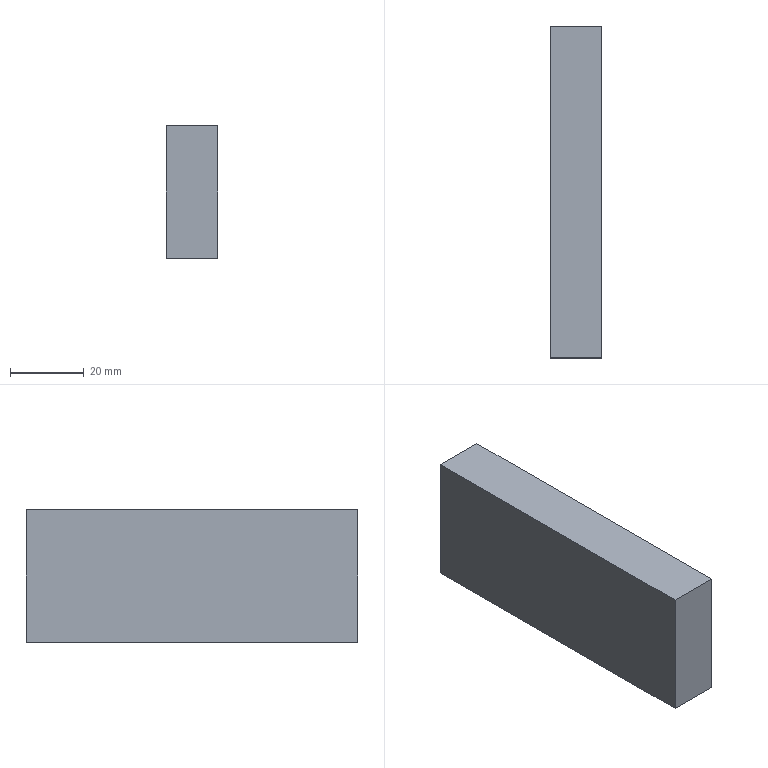Part | NX | features solid 2 | 1 solid | 6 faces | box 14 x 90 x 36 mm | volume 45360 mm3 | plane 6
STEP:
#1=CARTESIAN_POINT('',(300.,335.,9.));
#2=VERTEX_POINT('',#1);
#3=CARTESIAN_POINT('',(300.,245.,9.));
#4=VERTEX_POINT('',#3);
#5=CARTESIAN_POINT('',(300.,335.,9.));
#6=DIRECTION('',(0.,-1.,0.));
#7=VECTOR('',#6,1000.);
#8=LINE('',#5,#7);
#9=EDGE_CURVE('',#2,#4,#8,.T.);
#10=ORIENTED_EDGE('',*,*,#9,.T.);
#11=CARTESIAN_POINT('',(300.,245.,45.));
#12=VERTEX_POINT('',#11);
#13=CARTESIAN_POINT('',(300.,245.,45.));
#14=DIRECTION('',(0.,0.,-1.));
#15=VECTOR('',#14,1000.);
#16=LINE('',#13,#15);
#17=EDGE_CURVE('',#12,#4,#16,.T.);
#18=ORIENTED_EDGE('',*,*,#17,.F.);
#19=CARTESIAN_POINT('',(300.,335.,45.));
#20=VERTEX_POINT('',#19);
#21=CARTESIAN_POINT('',(300.,335.,45.));
#22=DIRECTION('',(0.,-1.,0.));
#23=VECTOR('',#22,1000.);
#24=LINE('',#21,#23);
#25=EDGE_CURVE('',#20,#12,#24,.T.);
#26=ORIENTED_EDGE('',*,*,#25,.F.);
#27=CARTESIAN_POINT('',(300.,335.,45.));
#28=DIRECTION('',(0.,0.,-1.));
#29=VECTOR('',#28,1000.);
#30=LINE('',#27,#29);
#31=EDGE_CURVE('',#20,#2,#30,.T.);
#32=ORIENTED_EDGE('',*,*,#31,.T.);
#33=EDGE_LOOP('',(#10,#18,#26,#32));
#34=FACE_BOUND('',#33,.T.);
#35=CARTESIAN_POINT('',(300.,335.,45.));
#36=DIRECTION('',(1.,0.,0.));
#37=DIRECTION('',(0.,0.,-1.));
#38=AXIS2_PLACEMENT_3D('',#35,#36,#37);
#39=PLANE('',#38);
#40=ADVANCED_FACE('',(#34),#39,.F.);
#41=CARTESIAN_POINT('',(314.,245.,9.));
#42=VERTEX_POINT('',#41);
#43=CARTESIAN_POINT('',(314.,245.,9.));
#44=DIRECTION('',(-1.,0.,0.));
#45=VECTOR('',#44,1000.);
#46=LINE('',#43,#45);
#47=EDGE_CURVE('',#42,#4,#46,.T.);
#48=ORIENTED_EDGE('',*,*,#47,.F.);
#49=CARTESIAN_POINT('',(314.,245.,45.));
#50=VERTEX_POINT('',#49);
#51=CARTESIAN_POINT('',(314.,245.,45.));
#52=DIRECTION('',(0.,0.,-1.));
#53=VECTOR('',#52,1000.);
#54=LINE('',#51,#53);
#55=EDGE_CURVE('',#50,#42,#54,.T.);
#56=ORIENTED_EDGE('',*,*,#55,.F.);
#57=CARTESIAN_POINT('',(314.,245.,45.));
#58=DIRECTION('',(-1.,0.,0.));
#59=VECTOR('',#58,1000.);
#60=LINE('',#57,#59);
#61=EDGE_CURVE('',#50,#12,#60,.T.);
#62=ORIENTED_EDGE('',*,*,#61,.T.);
#63=ORIENTED_EDGE('',*,*,#17,.T.);
#64=EDGE_LOOP('',(#48,#56,#62,#63));
#65=FACE_BOUND('',#64,.T.);
#66=CARTESIAN_POINT('',(314.,245.,45.));
#67=DIRECTION('',(0.,-1.,0.));
#68=DIRECTION('',(0.,0.,-1.));
#69=AXIS2_PLACEMENT_3D('',#66,#67,#68);
#70=PLANE('',#69);
#71=ADVANCED_FACE('',(#65),#70,.T.);
#72=CARTESIAN_POINT('',(314.,335.,9.));
#73=VERTEX_POINT('',#72);
#74=CARTESIAN_POINT('',(314.,335.,9.));
#75=DIRECTION('',(0.,-1.,0.));
#76=VECTOR('',#75,1000.);
#77=LINE('',#74,#76);
#78=EDGE_CURVE('',#73,#42,#77,.T.);
#79=ORIENTED_EDGE('',*,*,#78,.F.);
#80=CARTESIAN_POINT('',(314.,335.,45.));
#81=VERTEX_POINT('',#80);
#82=CARTESIAN_POINT('',(314.,335.,45.));
#83=DIRECTION('',(0.,0.,-1.));
#84=VECTOR('',#83,1000.);
#85=LINE('',#82,#84);
#86=EDGE_CURVE('',#81,#73,#85,.T.);
#87=ORIENTED_EDGE('',*,*,#86,.F.);
#88=CARTESIAN_POINT('',(314.,335.,45.));
#89=DIRECTION('',(0.,-1.,0.));
#90=VECTOR('',#89,1000.);
#91=LINE('',#88,#90);
#92=EDGE_CURVE('',#81,#50,#91,.T.);
#93=ORIENTED_EDGE('',*,*,#92,.T.);
#94=ORIENTED_EDGE('',*,*,#55,.T.);
#95=EDGE_LOOP('',(#79,#87,#93,#94));
#96=FACE_BOUND('',#95,.T.);
#97=CARTESIAN_POINT('',(314.,335.,45.));
#98=DIRECTION('',(1.,0.,0.));
#99=DIRECTION('',(0.,0.,-1.));
#100=AXIS2_PLACEMENT_3D('',#97,#98,#99);
#101=PLANE('',#100);
#102=ADVANCED_FACE('',(#96),#101,.T.);
#103=CARTESIAN_POINT('',(314.,335.,9.));
#104=DIRECTION('',(-1.,0.,0.));
#105=VECTOR('',#104,1000.);
#106=LINE('',#103,#105);
#107=EDGE_CURVE('',#73,#2,#106,.T.);
#108=ORIENTED_EDGE('',*,*,#107,.T.);
#109=ORIENTED_EDGE('',*,*,#31,.F.);
#110=CARTESIAN_POINT('',(314.,335.,45.));
#111=DIRECTION('',(-1.,0.,0.));
#112=VECTOR('',#111,1000.);
#113=LINE('',#110,#112);
#114=EDGE_CURVE('',#81,#20,#113,.T.);
#115=ORIENTED_EDGE('',*,*,#114,.F.);
#116=ORIENTED_EDGE('',*,*,#86,.T.);
#117=EDGE_LOOP('',(#108,#109,#115,#116));
#118=FACE_BOUND('',#117,.T.);
#119=CARTESIAN_POINT('',(314.,335.,45.));
#120=DIRECTION('',(0.,-1.,0.));
#121=DIRECTION('',(0.,0.,-1.));
#122=AXIS2_PLACEMENT_3D('',#119,#120,#121);
#123=PLANE('',#122);
#124=ADVANCED_FACE('',(#118),#123,.F.);
#125=ORIENTED_EDGE('',*,*,#25,.T.);
#126=ORIENTED_EDGE('',*,*,#61,.F.);
#127=ORIENTED_EDGE('',*,*,#92,.F.);
#128=ORIENTED_EDGE('',*,*,#114,.T.);
#129=EDGE_LOOP('',(#125,#126,#127,#128));
#130=FACE_BOUND('',#129,.T.);
#131=CARTESIAN_POINT('',(300.,245.,45.));
#132=DIRECTION('',(0.,0.,-1.));
#133=DIRECTION('',(-1.,0.,0.));
#134=AXIS2_PLACEMENT_3D('',#131,#132,#133);
#135=PLANE('',#134);
#136=ADVANCED_FACE('',(#130),#135,.F.);
#137=ORIENTED_EDGE('',*,*,#9,.F.);
#138=ORIENTED_EDGE('',*,*,#107,.F.);
#139=ORIENTED_EDGE('',*,*,#78,.T.);
#140=ORIENTED_EDGE('',*,*,#47,.T.);
#141=EDGE_LOOP('',(#137,#138,#139,#140));
#142=FACE_BOUND('',#141,.T.);
#143=CARTESIAN_POINT('',(300.,245.,9.));
#144=DIRECTION('',(0.,0.,-1.));
#145=DIRECTION('',(-1.,0.,0.));
#146=AXIS2_PLACEMENT_3D('',#143,#144,#145);
#147=PLANE('',#146);
#148=ADVANCED_FACE('',(#142),#147,.T.);
#149=CLOSED_SHELL('',(#40,#71,#102,#124,#136,#148));
#150=MANIFOLD_SOLID_BREP('',#149);
#151=(LENGTH_UNIT()NAMED_UNIT(*)SI_UNIT(.MILLI.,.METRE.));
#152=UNCERTAINTY_MEASURE_WITH_UNIT(LENGTH_MEASURE(0.00001),#151,'','');
#153=(NAMED_UNIT(*)PLANE_ANGLE_UNIT()SI_UNIT($,.RADIAN.));
#154=(NAMED_UNIT(*)SI_UNIT($,.STERADIAN.)SOLID_ANGLE_UNIT());
#155=(GEOMETRIC_REPRESENTATION_CONTEXT(3)GLOBAL_UNCERTAINTY_ASSIGNED_CONTEXT((#152))GLOBAL_UNIT_ASSIGNED_CONTEXT((#151,#153,#154))REPRESENTATION_CONTEXT('',''));
#156=ADVANCED_BREP_SHAPE_REPRESENTATION('',(#150),#155);